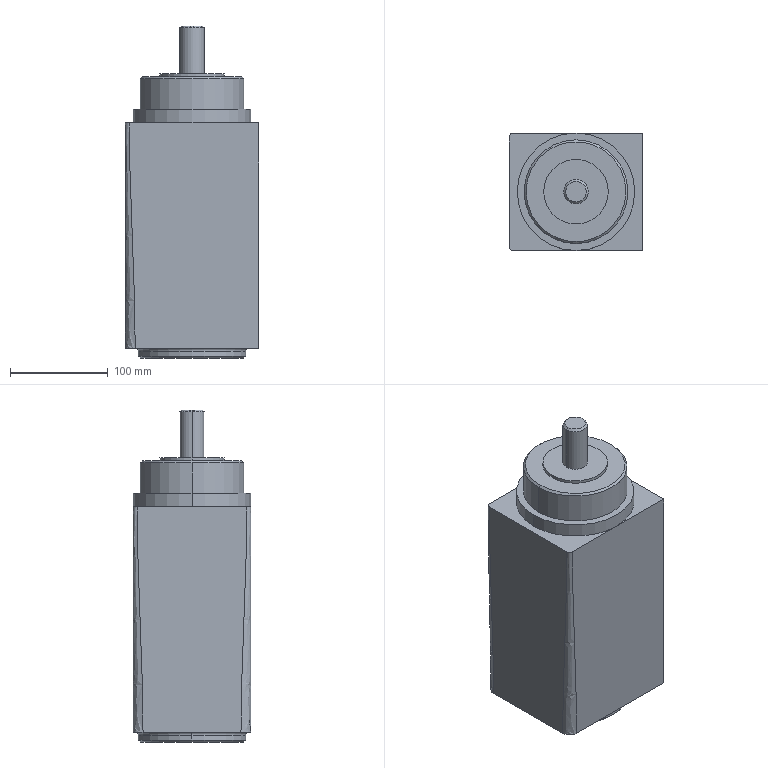Part | SolidWorks | features ICE 5, Chamfer 3, Extrusion 1, Fillet 1, VarFillet 1 | 1 solid | 32 faces | box 136 x 120 x 339 mm | volume 4326420 mm3 | plane 12 | cylinder 10 | cone 6 | torus 2 | spline 2 | commonest cylinder face diameters 25 x2 66 x2 106 x2 110 x2 120 x2
STEP:
#1=CARTESIAN_POINT('',(-53.,1.606,-240.));
#2=VERTEX_POINT('',#1);
#3=CARTESIAN_POINT('',(53.,1.606,-240.));
#4=VERTEX_POINT('',#3);
#5=CARTESIAN_POINT('',(0.,1.606,-240.));
#6=DIRECTION('',(0.,0.,-1.));
#7=DIRECTION('',(-1.,0.,0.));
#8=AXIS2_PLACEMENT_3D('',#5,#6,#7);
#9=CIRCLE('',#8,53.);
#10=EDGE_CURVE('',#2,#4,#9,.T.);
#11=ORIENTED_EDGE('',*,*,#10,.F.);
#12=CARTESIAN_POINT('',(-55.,1.606,-238.));
#13=VERTEX_POINT('',#12);
#14=CARTESIAN_POINT('',(-53.,1.606,-240.));
#15=DIRECTION('',(-0.7071,0.,0.7071));
#16=VECTOR('',#15,1000.);
#17=LINE('',#14,#16);
#18=EDGE_CURVE('',#2,#13,#17,.T.);
#19=ORIENTED_EDGE('',*,*,#18,.T.);
#20=CARTESIAN_POINT('',(55.,1.606,-238.));
#21=VERTEX_POINT('',#20);
#22=CARTESIAN_POINT('',(0.,1.606,-238.));
#23=DIRECTION('',(0.,0.,1.));
#24=DIRECTION('',(-1.,0.,0.));
#25=AXIS2_PLACEMENT_3D('',#22,#23,#24);
#26=CIRCLE('',#25,55.);
#27=EDGE_CURVE('',#21,#13,#26,.T.);
#28=ORIENTED_EDGE('',*,*,#27,.F.);
#29=CARTESIAN_POINT('',(53.,1.606,-240.));
#30=DIRECTION('',(0.7071,0.,0.7071));
#31=VECTOR('',#30,1000.);
#32=LINE('',#29,#31);
#33=EDGE_CURVE('',#4,#21,#32,.T.);
#34=ORIENTED_EDGE('',*,*,#33,.F.);
#35=EDGE_LOOP('',(#11,#19,#28,#34));
#36=FACE_OUTER_BOUND('',#35,.T.);
#37=CARTESIAN_POINT('',(0.,1.606,-240.));
#38=DIRECTION('',(0.,0.,1.));
#39=DIRECTION('',(1.,0.,0.));
#40=AXIS2_PLACEMENT_3D('',#37,#38,#39);
#41=CONICAL_SURFACE('',#40,53.,0.7854);
#42=ADVANCED_FACE('',(#36),#41,.T.);
#43=CARTESIAN_POINT('',(51.,1.606,47.));
#44=VERTEX_POINT('',#43);
#45=CARTESIAN_POINT('',(-51.,1.606,47.));
#46=VERTEX_POINT('',#45);
#47=CARTESIAN_POINT('',(0.,1.606,47.));
#48=DIRECTION('',(0.,0.,1.));
#49=DIRECTION('',(1.,0.,0.));
#50=AXIS2_PLACEMENT_3D('',#47,#48,#49);
#51=CIRCLE('',#50,51.);
#52=EDGE_CURVE('',#44,#46,#51,.T.);
#53=ORIENTED_EDGE('',*,*,#52,.F.);
#54=CARTESIAN_POINT('',(53.,1.606,45.));
#55=VERTEX_POINT('',#54);
#56=CARTESIAN_POINT('',(51.,1.606,47.));
#57=DIRECTION('',(0.7071,0.,-0.7071));
#58=VECTOR('',#57,1000.);
#59=LINE('',#56,#58);
#60=EDGE_CURVE('',#44,#55,#59,.T.);
#61=ORIENTED_EDGE('',*,*,#60,.T.);
#62=CARTESIAN_POINT('',(-53.,1.606,45.));
#63=VERTEX_POINT('',#62);
#64=CARTESIAN_POINT('',(0.,1.606,45.));
#65=DIRECTION('',(0.,0.,-1.));
#66=DIRECTION('',(1.,0.,0.));
#67=AXIS2_PLACEMENT_3D('',#64,#65,#66);
#68=CIRCLE('',#67,53.);
#69=EDGE_CURVE('',#63,#55,#68,.T.);
#70=ORIENTED_EDGE('',*,*,#69,.F.);
#71=CARTESIAN_POINT('',(-51.,1.606,47.));
#72=DIRECTION('',(-0.7071,0.,-0.7071));
#73=VECTOR('',#72,1000.);
#74=LINE('',#71,#73);
#75=EDGE_CURVE('',#46,#63,#74,.T.);
#76=ORIENTED_EDGE('',*,*,#75,.F.);
#77=EDGE_LOOP('',(#53,#61,#70,#76));
#78=FACE_OUTER_BOUND('',#77,.T.);
#79=CARTESIAN_POINT('',(0.,1.606,47.));
#80=DIRECTION('',(0.,0.,-1.));
#81=DIRECTION('',(-1.,0.,0.));
#82=AXIS2_PLACEMENT_3D('',#79,#80,#81);
#83=CONICAL_SURFACE('',#82,51.,0.7854);
#84=ADVANCED_FACE('',(#78),#83,.T.);
#85=CARTESIAN_POINT('',(-58.,1.606,-230.));
#86=VERTEX_POINT('',#85);
#87=CARTESIAN_POINT('',(58.,1.606,-230.));
#88=VERTEX_POINT('',#87);
#89=CARTESIAN_POINT('',(0.,1.606,-230.));
#90=DIRECTION('',(0.,0.,1.));
#91=DIRECTION('',(1.,0.,0.));
#92=AXIS2_PLACEMENT_3D('',#89,#90,#91);
#93=CIRCLE('',#92,58.);
#94=EDGE_CURVE('',#86,#88,#93,.T.);
#95=ORIENTED_EDGE('',*,*,#94,.F.);
#96=CARTESIAN_POINT('',(-55.,1.606,-233.));
#97=VERTEX_POINT('',#96);
#98=CARTESIAN_POINT('',(-58.,1.606,-233.));
#99=DIRECTION('',(0.,1.,0.));
#100=DIRECTION('',(-1.,0.,0.));
#101=AXIS2_PLACEMENT_3D('',#98,#99,#100);
#102=CIRCLE('',#101,3.);
#103=EDGE_CURVE('',#86,#97,#102,.T.);
#104=ORIENTED_EDGE('',*,*,#103,.T.);
#105=CARTESIAN_POINT('',(55.,1.606,-233.));
#106=VERTEX_POINT('',#105);
#107=CARTESIAN_POINT('',(0.,1.606,-233.));
#108=DIRECTION('',(0.,0.,-1.));
#109=DIRECTION('',(1.,0.,0.));
#110=AXIS2_PLACEMENT_3D('',#107,#108,#109);
#111=CIRCLE('',#110,55.);
#112=EDGE_CURVE('',#106,#97,#111,.T.);
#113=ORIENTED_EDGE('',*,*,#112,.F.);
#114=CARTESIAN_POINT('',(58.,1.606,-233.));
#115=DIRECTION('',(0.,-1.,0.));
#116=DIRECTION('',(0.,0.,-1.));
#117=AXIS2_PLACEMENT_3D('',#114,#115,#116);
#118=CIRCLE('',#117,3.);
#119=EDGE_CURVE('',#88,#106,#118,.T.);
#120=ORIENTED_EDGE('',*,*,#119,.F.);
#121=EDGE_LOOP('',(#95,#104,#113,#120));
#122=FACE_OUTER_BOUND('',#121,.T.);
#123=CARTESIAN_POINT('',(0.,1.606,-233.));
#124=DIRECTION('',(0.,0.,1.));
#125=DIRECTION('',(1.,0.,0.));
#126=AXIS2_PLACEMENT_3D('',#123,#124,#125);
#127=TOROIDAL_SURFACE('',#126,58.,3.);
#128=ADVANCED_FACE('',(#122),#127,.F.);
#129=ORIENTED_EDGE('',*,*,#27,.T.);
#130=CARTESIAN_POINT('',(-55.,1.606,-240.));
#131=DIRECTION('',(0.,0.,1.));
#132=VECTOR('',#131,1000.);
#133=LINE('',#130,#132);
#134=EDGE_CURVE('',#13,#97,#133,.T.);
#135=ORIENTED_EDGE('',*,*,#134,.T.);
#136=CARTESIAN_POINT('',(0.,1.606,-233.));
#137=DIRECTION('',(0.,0.,-1.));
#138=DIRECTION('',(1.,0.,0.));
#139=AXIS2_PLACEMENT_3D('',#136,#137,#138);
#140=CIRCLE('',#139,55.);
#141=EDGE_CURVE('',#97,#106,#140,.T.);
#142=ORIENTED_EDGE('',*,*,#141,.T.);
#143=CARTESIAN_POINT('',(55.,1.606,-240.));
#144=DIRECTION('',(0.,0.,1.));
#145=VECTOR('',#144,1000.);
#146=LINE('',#143,#145);
#147=EDGE_CURVE('',#21,#106,#146,.T.);
#148=ORIENTED_EDGE('',*,*,#147,.F.);
#149=EDGE_LOOP('',(#129,#135,#142,#148));
#150=FACE_OUTER_BOUND('',#149,.T.);
#151=CARTESIAN_POINT('',(0.,1.606,-240.));
#152=DIRECTION('',(0.,0.,1.));
#153=DIRECTION('',(1.,0.,0.));
#154=AXIS2_PLACEMENT_3D('',#151,#152,#153);
#155=CYLINDRICAL_SURFACE('',#154,55.);
#156=ADVANCED_FACE('',(#150),#155,.T.);
#157=CARTESIAN_POINT('',(10.5,1.606,99.));
#158=VERTEX_POINT('',#157);
#159=CARTESIAN_POINT('',(-10.5,1.606,99.));
#160=VERTEX_POINT('',#159);
#161=CARTESIAN_POINT('',(0.,1.606,99.));
#162=DIRECTION('',(0.,0.,1.));
#163=DIRECTION('',(1.,0.,0.));
#164=AXIS2_PLACEMENT_3D('',#161,#162,#163);
#165=CIRCLE('',#164,10.5);
#166=EDGE_CURVE('',#158,#160,#165,.T.);
#167=ORIENTED_EDGE('',*,*,#166,.F.);
#168=CARTESIAN_POINT('',(12.5,1.606,97.));
#169=VERTEX_POINT('',#168);
#170=CARTESIAN_POINT('',(10.5,1.606,99.));
#171=DIRECTION('',(0.7071,0.,-0.7071));
#172=VECTOR('',#171,1000.);
#173=LINE('',#170,#172);
#174=EDGE_CURVE('',#158,#169,#173,.T.);
#175=ORIENTED_EDGE('',*,*,#174,.T.);
#176=CARTESIAN_POINT('',(-12.5,1.606,97.));
#177=VERTEX_POINT('',#176);
#178=CARTESIAN_POINT('',(0.,1.606,97.));
#179=DIRECTION('',(0.,0.,-1.));
#180=DIRECTION('',(1.,0.,0.));
#181=AXIS2_PLACEMENT_3D('',#178,#179,#180);
#182=CIRCLE('',#181,12.5);
#183=EDGE_CURVE('',#177,#169,#182,.T.);
#184=ORIENTED_EDGE('',*,*,#183,.F.);
#185=CARTESIAN_POINT('',(-10.5,1.606,99.));
#186=DIRECTION('',(-0.7071,0.,-0.7071));
#187=VECTOR('',#186,1000.);
#188=LINE('',#185,#187);
#189=EDGE_CURVE('',#160,#177,#188,.T.);
#190=ORIENTED_EDGE('',*,*,#189,.F.);
#191=EDGE_LOOP('',(#167,#175,#184,#190));
#192=FACE_OUTER_BOUND('',#191,.T.);
#193=CARTESIAN_POINT('',(0.,1.606,99.));
#194=DIRECTION('',(0.,0.,-1.));
#195=DIRECTION('',(-1.,0.,0.));
#196=AXIS2_PLACEMENT_3D('',#193,#194,#195);
#197=CONICAL_SURFACE('',#196,10.5,0.7854);
#198=ADVANCED_FACE('',(#192),#197,.T.);
#199=ORIENTED_EDGE('',*,*,#183,.T.);
#200=CARTESIAN_POINT('',(12.5,1.606,50.));
#201=VERTEX_POINT('',#200);
#202=CARTESIAN_POINT('',(12.5,1.606,99.));
#203=DIRECTION('',(0.,0.,-1.));
#204=VECTOR('',#203,1000.);
#205=LINE('',#202,#204);
#206=EDGE_CURVE('',#169,#201,#205,.T.);
#207=ORIENTED_EDGE('',*,*,#206,.T.);
#208=CARTESIAN_POINT('',(-12.5,1.606,50.));
#209=VERTEX_POINT('',#208);
#210=CARTESIAN_POINT('',(0.,1.606,50.));
#211=DIRECTION('',(0.,0.,1.));
#212=DIRECTION('',(1.,0.,0.));
#213=AXIS2_PLACEMENT_3D('',#210,#211,#212);
#214=CIRCLE('',#213,12.5);
#215=EDGE_CURVE('',#201,#209,#214,.T.);
#216=ORIENTED_EDGE('',*,*,#215,.T.);
#217=CARTESIAN_POINT('',(-12.5,1.606,99.));
#218=DIRECTION('',(0.,0.,-1.));
#219=VECTOR('',#218,1000.);
#220=LINE('',#217,#219);
#221=EDGE_CURVE('',#177,#209,#220,.T.);
#222=ORIENTED_EDGE('',*,*,#221,.F.);
#223=EDGE_LOOP('',(#199,#207,#216,#222));
#224=FACE_OUTER_BOUND('',#223,.T.);
#225=CARTESIAN_POINT('',(0.,1.606,99.));
#226=DIRECTION('',(0.,0.,-1.));
#227=DIRECTION('',(-1.,0.,0.));
#228=AXIS2_PLACEMENT_3D('',#225,#226,#227);
#229=CYLINDRICAL_SURFACE('',#228,12.5);
#230=ADVANCED_FACE('',(#224),#229,.T.);
#231=CARTESIAN_POINT('',(33.,1.606,50.));
#232=VERTEX_POINT('',#231);
#233=CARTESIAN_POINT('',(-33.,1.606,50.));
#234=VERTEX_POINT('',#233);
#235=CARTESIAN_POINT('',(0.,1.606,50.));
#236=DIRECTION('',(0.,0.,1.));
#237=DIRECTION('',(1.,0.,0.));
#238=AXIS2_PLACEMENT_3D('',#235,#236,#237);
#239=CIRCLE('',#238,33.);
#240=EDGE_CURVE('',#232,#234,#239,.T.);
#241=ORIENTED_EDGE('',*,*,#240,.F.);
#242=CARTESIAN_POINT('',(33.,1.606,47.));
#243=VERTEX_POINT('',#242);
#244=CARTESIAN_POINT('',(33.,1.606,50.));
#245=DIRECTION('',(0.,0.,-1.));
#246=VECTOR('',#245,1000.);
#247=LINE('',#244,#246);
#248=EDGE_CURVE('',#232,#243,#247,.T.);
#249=ORIENTED_EDGE('',*,*,#248,.T.);
#250=CARTESIAN_POINT('',(-33.,1.606,47.));
#251=VERTEX_POINT('',#250);
#252=CARTESIAN_POINT('',(0.,1.606,47.));
#253=DIRECTION('',(0.,0.,1.));
#254=DIRECTION('',(1.,0.,0.));
#255=AXIS2_PLACEMENT_3D('',#252,#253,#254);
#256=CIRCLE('',#255,33.);
#257=EDGE_CURVE('',#243,#251,#256,.T.);
#258=ORIENTED_EDGE('',*,*,#257,.T.);
#259=CARTESIAN_POINT('',(-33.,1.606,50.));
#260=DIRECTION('',(0.,0.,-1.));
#261=VECTOR('',#260,1000.);
#262=LINE('',#259,#261);
#263=EDGE_CURVE('',#234,#251,#262,.T.);
#264=ORIENTED_EDGE('',*,*,#263,.F.);
#265=EDGE_LOOP('',(#241,#249,#258,#264));
#266=FACE_OUTER_BOUND('',#265,.T.);
#267=CARTESIAN_POINT('',(0.,1.606,50.));
#268=DIRECTION('',(0.,0.,-1.));
#269=DIRECTION('',(-1.,0.,0.));
#270=AXIS2_PLACEMENT_3D('',#267,#268,#269);
#271=CYLINDRICAL_SURFACE('',#270,33.);
#272=ADVANCED_FACE('',(#266),#271,.T.);
#273=ORIENTED_EDGE('',*,*,#69,.T.);
#274=CARTESIAN_POINT('',(53.,1.606,14.));
#275=VERTEX_POINT('',#274);
#276=CARTESIAN_POINT('',(53.,1.606,47.));
#277=DIRECTION('',(0.,0.,-1.));
#278=VECTOR('',#277,1000.);
#279=LINE('',#276,#278);
#280=EDGE_CURVE('',#55,#275,#279,.T.);
#281=ORIENTED_EDGE('',*,*,#280,.T.);
#282=CARTESIAN_POINT('',(-53.,1.606,14.));
#283=VERTEX_POINT('',#282);
#284=CARTESIAN_POINT('',(0.,1.606,14.));
#285=DIRECTION('',(0.,0.,1.));
#286=DIRECTION('',(1.,0.,0.));
#287=AXIS2_PLACEMENT_3D('',#284,#285,#286);
#288=CIRCLE('',#287,53.);
#289=EDGE_CURVE('',#275,#283,#288,.T.);
#290=ORIENTED_EDGE('',*,*,#289,.T.);
#291=CARTESIAN_POINT('',(-53.,1.606,47.));
#292=DIRECTION('',(0.,0.,-1.));
#293=VECTOR('',#292,1000.);
#294=LINE('',#291,#293);
#295=EDGE_CURVE('',#63,#283,#294,.T.);
#296=ORIENTED_EDGE('',*,*,#295,.F.);
#297=EDGE_LOOP('',(#273,#281,#290,#296));
#298=FACE_OUTER_BOUND('',#297,.T.);
#299=CARTESIAN_POINT('',(0.,1.606,47.));
#300=DIRECTION('',(0.,0.,-1.));
#301=DIRECTION('',(-1.,0.,0.));
#302=AXIS2_PLACEMENT_3D('',#299,#300,#301);
#303=CYLINDRICAL_SURFACE('',#302,53.);
#304=ADVANCED_FACE('',(#298),#303,.T.);
#305=CARTESIAN_POINT('',(60.,1.606,14.));
#306=VERTEX_POINT('',#305);
#307=CARTESIAN_POINT('',(-60.,1.606,14.));
#308=VERTEX_POINT('',#307);
#309=CARTESIAN_POINT('',(0.,1.606,14.));
#310=DIRECTION('',(0.,0.,1.));
#311=DIRECTION('',(1.,0.,0.));
#312=AXIS2_PLACEMENT_3D('',#309,#310,#311);
#313=CIRCLE('',#312,60.);
#314=EDGE_CURVE('',#306,#308,#313,.T.);
#315=ORIENTED_EDGE('',*,*,#314,.F.);
#316=CARTESIAN_POINT('',(60.,1.606,0.));
#317=VERTEX_POINT('',#316);
#318=CARTESIAN_POINT('',(60.,1.606,14.));
#319=DIRECTION('',(0.,0.,-1.));
#320=VECTOR('',#319,1000.);
#321=LINE('',#318,#320);
#322=EDGE_CURVE('',#306,#317,#321,.T.);
#323=ORIENTED_EDGE('',*,*,#322,.T.);
#324=CARTESIAN_POINT('',(0.,61.606,0.));
#325=VERTEX_POINT('',#324);
#326=CARTESIAN_POINT('',(0.,1.606,0.));
#327=DIRECTION('',(0.,0.,1.));
#328=DIRECTION('',(1.,0.,0.));
#329=AXIS2_PLACEMENT_3D('',#326,#327,#328);
#330=CIRCLE('',#329,60.);
#331=EDGE_CURVE('',#317,#325,#330,.T.);
#332=ORIENTED_EDGE('',*,*,#331,.T.);
#333=CARTESIAN_POINT('',(-60.,1.606,0.));
#334=VERTEX_POINT('',#333);
#335=CARTESIAN_POINT('',(0.,1.606,0.));
#336=DIRECTION('',(0.,0.,1.));
#337=DIRECTION('',(1.,0.,0.));
#338=AXIS2_PLACEMENT_3D('',#335,#336,#337);
#339=CIRCLE('',#338,60.);
#340=EDGE_CURVE('',#325,#334,#339,.T.);
#341=ORIENTED_EDGE('',*,*,#340,.T.);
#342=CARTESIAN_POINT('',(-60.,1.606,14.));
#343=DIRECTION('',(0.,0.,-1.));
#344=VECTOR('',#343,1000.);
#345=LINE('',#342,#344);
#346=EDGE_CURVE('',#308,#334,#345,.T.);
#347=ORIENTED_EDGE('',*,*,#346,.F.);
#348=EDGE_LOOP('',(#315,#323,#332,#341,#347));
#349=FACE_OUTER_BOUND('',#348,.T.);
#350=CARTESIAN_POINT('',(0.,1.606,14.));
#351=DIRECTION('',(0.,0.,-1.));
#352=DIRECTION('',(-1.,0.,0.));
#353=AXIS2_PLACEMENT_3D('',#350,#351,#352);
#354=CYLINDRICAL_SURFACE('',#353,60.);
#355=ADVANCED_FACE('',(#349),#354,.T.);
#356=CARTESIAN_POINT('',(-68.,57.606,0.));
#357=VERTEX_POINT('',#356);
#358=CARTESIAN_POINT('',(-68.,-54.394,0.));
#359=VERTEX_POINT('',#358);
#360=CARTESIAN_POINT('',(-68.,61.606,0.));
#361=DIRECTION('',(0.,-1.,0.));
#362=VECTOR('',#361,1000.);
#363=LINE('',#360,#362);
#364=EDGE_CURVE('',#357,#359,#363,.T.);
#365=ORIENTED_EDGE('',*,*,#364,.T.);
#366=CARTESIAN_POINT('',(-64.,-58.394,0.));
#367=VERTEX_POINT('',#366);
#368=CARTESIAN_POINT('',(-68.,-54.394,0.));
#369=CARTESIAN_POINT('',(-68.,-58.394,0.));
#370=CARTESIAN_POINT('',(-64.,-58.394,0.));
#371=(BOUNDED_CURVE()B_SPLINE_CURVE(2,(#368,#369,#370),.UNSPECIFIED.,.F.,.F.)B_SPLINE_CURVE_WITH_KNOTS((3,3),(0.,0.006249),.UNSPECIFIED.)CURVE()GEOMETRIC_REPRESENTATION_ITEM()RATIONAL_B_SPLINE_CURVE((1.,0.7071,1.))REPRESENTATION_ITEM(''));
#372=EDGE_CURVE('',#359,#367,#371,.T.);
#373=ORIENTED_EDGE('',*,*,#372,.T.);
#374=CARTESIAN_POINT('',(0.,-58.394,0.));
#375=VERTEX_POINT('',#374);
#376=CARTESIAN_POINT('',(-68.,-58.394,0.));
#377=DIRECTION('',(1.,0.,0.));
#378=VECTOR('',#377,1000.);
#379=LINE('',#376,#378);
#380=EDGE_CURVE('',#367,#375,#379,.T.);
#381=ORIENTED_EDGE('',*,*,#380,.T.);
#382=CARTESIAN_POINT('',(0.,1.606,0.));
#383=DIRECTION('',(0.,0.,1.));
#384=DIRECTION('',(1.,0.,0.));
#385=AXIS2_PLACEMENT_3D('',#382,#383,#384);
#386=CIRCLE('',#385,60.);
#387=EDGE_CURVE('',#334,#375,#386,.T.);
#388=ORIENTED_EDGE('',*,*,#387,.F.);
#389=ORIENTED_EDGE('',*,*,#340,.F.);
#390=CARTESIAN_POINT('',(-64.,61.606,0.));
#391=VERTEX_POINT('',#390);
#392=CARTESIAN_POINT('',(-68.,61.606,0.));
#393=DIRECTION('',(1.,0.,0.));
#394=VECTOR('',#393,1000.);
#395=LINE('',#392,#394);
#396=EDGE_CURVE('',#391,#325,#395,.T.);
#397=ORIENTED_EDGE('',*,*,#396,.F.);
#398=CARTESIAN_POINT('',(-64.,61.606,0.));
#399=CARTESIAN_POINT('',(-68.,61.606,0.));
#400=CARTESIAN_POINT('',(-68.,57.606,0.));
#401=(BOUNDED_CURVE()B_SPLINE_CURVE(2,(#398,#399,#400),.UNSPECIFIED.,.F.,.T.)B_SPLINE_CURVE_WITH_KNOTS((3,3),(0.,0.006249),.UNSPECIFIED.)CURVE()GEOMETRIC_REPRESENTATION_ITEM()RATIONAL_B_SPLINE_CURVE((1.,0.7071,1.))REPRESENTATION_ITEM(''));
#402=EDGE_CURVE('',#391,#357,#401,.T.);
#403=ORIENTED_EDGE('',*,*,#402,.T.);
#404=EDGE_LOOP('',(#365,#373,#381,#388,#389,#397,#403));
#405=FACE_OUTER_BOUND('',#404,.T.);
#406=CARTESIAN_POINT('',(0.,0.,0.));
#407=DIRECTION('',(0.,0.,1.));
#408=DIRECTION('',(1.,0.,0.));
#409=AXIS2_PLACEMENT_3D('',#406,#407,#408);
#410=PLANE('',#409);
#411=ADVANCED_FACE('',(#405),#410,.T.);
#412=CARTESIAN_POINT('',(-68.,51.606,-230.));
#413=VERTEX_POINT('',#412);
#414=CARTESIAN_POINT('',(-68.,-48.394,-230.));
#415=VERTEX_POINT('',#414);
#416=CARTESIAN_POINT('',(-68.,61.606,-230.));
#417=DIRECTION('',(0.,-1.,0.));
#418=VECTOR('',#417,1000.);
#419=LINE('',#416,#418);
#420=EDGE_CURVE('',#413,#415,#419,.T.);
#421=ORIENTED_EDGE('',*,*,#420,.T.);
#422=CARTESIAN_POINT('',(-68.,-48.394,-230.));
#423=CARTESIAN_POINT('',(-68.,-48.394,-153.333));
#424=CARTESIAN_POINT('',(-68.,-54.394,-76.667));
#425=CARTESIAN_POINT('',(-68.,-54.394,0.));
#426=B_SPLINE_CURVE_WITH_KNOTS('',3,(#422,#423,#424,#425),.UNSPECIFIED.,.F.,.F.,(4,4),(0.,0.23),.UNSPECIFIED.);
#427=EDGE_CURVE('',#415,#359,#426,.T.);
#428=ORIENTED_EDGE('',*,*,#427,.T.);
#429=ORIENTED_EDGE('',*,*,#364,.F.);
#430=CARTESIAN_POINT('',(-68.,57.606,0.));
#431=CARTESIAN_POINT('',(-68.,57.606,-76.667));
#432=CARTESIAN_POINT('',(-68.,51.606,-153.333));
#433=CARTESIAN_POINT('',(-68.,51.606,-230.));
#434=B_SPLINE_CURVE_WITH_KNOTS('',3,(#430,#431,#432,#433),.UNSPECIFIED.,.F.,.F.,(4,4),(0.,0.23),.UNSPECIFIED.);
#435=EDGE_CURVE('',#357,#413,#434,.T.);
#436=ORIENTED_EDGE('',*,*,#435,.T.);
#437=EDGE_LOOP('',(#421,#428,#429,#436));
#438=FACE_OUTER_BOUND('',#437,.T.);
#439=CARTESIAN_POINT('',(-68.,61.606,-230.));
#440=DIRECTION('',(-1.,0.,0.));
#441=DIRECTION('',(0.,0.,1.));
#442=AXIS2_PLACEMENT_3D('',#439,#440,#441);
#443=PLANE('',#442);
#444=ADVANCED_FACE('',(#438),#443,.T.);
#445=CARTESIAN_POINT('',(-58.,61.606,-230.));
#446=VERTEX_POINT('',#445);
#447=CARTESIAN_POINT('',(68.,61.606,-230.));
#448=VERTEX_POINT('',#447);
#449=CARTESIAN_POINT('',(-68.,61.606,-230.));
#450=DIRECTION('',(1.,0.,0.));
#451=VECTOR('',#450,1000.);
#452=LINE('',#449,#451);
#453=EDGE_CURVE('',#446,#448,#452,.T.);
#454=ORIENTED_EDGE('',*,*,#453,.F.);
#455=CARTESIAN_POINT('',(-58.,61.606,-230.));
#456=CARTESIAN_POINT('',(-58.,61.606,-153.333));
#457=CARTESIAN_POINT('',(-64.,61.606,-76.667));
#458=CARTESIAN_POINT('',(-64.,61.606,0.));
#459=B_SPLINE_CURVE_WITH_KNOTS('',3,(#455,#456,#457,#458),.UNSPECIFIED.,.F.,.F.,(4,4),(0.,0.23),.UNSPECIFIED.);
#460=EDGE_CURVE('',#446,#391,#459,.T.);
#461=ORIENTED_EDGE('',*,*,#460,.T.);
#462=ORIENTED_EDGE('',*,*,#396,.T.);
#463=CARTESIAN_POINT('',(68.,61.606,0.));
#464=VERTEX_POINT('',#463);
#465=CARTESIAN_POINT('',(-68.,61.606,0.));
#466=DIRECTION('',(1.,0.,0.));
#467=VECTOR('',#466,1000.);
#468=LINE('',#465,#467);
#469=EDGE_CURVE('',#325,#464,#468,.T.);
#470=ORIENTED_EDGE('',*,*,#469,.T.);
#471=CARTESIAN_POINT('',(68.,61.606,-230.));
#472=DIRECTION('',(0.,0.,1.));
#473=VECTOR('',#472,1000.);
#474=LINE('',#471,#473);
#475=EDGE_CURVE('',#448,#464,#474,.T.);
#476=ORIENTED_EDGE('',*,*,#475,.F.);
#477=EDGE_LOOP('',(#454,#461,#462,#470,#476));
#478=FACE_OUTER_BOUND('',#477,.T.);
#479=CARTESIAN_POINT('',(-68.,61.606,-230.));
#480=DIRECTION('',(0.,-1.,0.));
#481=DIRECTION('',(1.,0.,0.));
#482=AXIS2_PLACEMENT_3D('',#479,#480,#481);
#483=PLANE('',#482);
#484=ADVANCED_FACE('',(#478),#483,.F.);
#485=CARTESIAN_POINT('',(68.,-58.394,0.));
#486=VERTEX_POINT('',#485);
#487=CARTESIAN_POINT('',(68.,61.606,0.));
#488=DIRECTION('',(0.,-1.,0.));
#489=VECTOR('',#488,1000.);
#490=LINE('',#487,#489);
#491=EDGE_CURVE('',#464,#486,#490,.T.);
#492=ORIENTED_EDGE('',*,*,#491,.T.);
#493=CARTESIAN_POINT('',(68.,-58.394,-230.));
#494=VERTEX_POINT('',#493);
#495=CARTESIAN_POINT('',(68.,-58.394,-230.));
#496=DIRECTION('',(0.,0.,1.));
#497=VECTOR('',#496,1000.);
#498=LINE('',#495,#497);
#499=EDGE_CURVE('',#494,#486,#498,.T.);
#500=ORIENTED_EDGE('',*,*,#499,.F.);
#501=CARTESIAN_POINT('',(68.,61.606,-230.));
#502=DIRECTION('',(0.,-1.,0.));
#503=VECTOR('',#502,1000.);
#504=LINE('',#501,#503);
#505=EDGE_CURVE('',#448,#494,#504,.T.);
#506=ORIENTED_EDGE('',*,*,#505,.F.);
#507=ORIENTED_EDGE('',*,*,#475,.T.);
#508=EDGE_LOOP('',(#492,#500,#506,#507));
#509=FACE_OUTER_BOUND('',#508,.T.);
#510=CARTESIAN_POINT('',(68.,61.606,-230.));
#511=DIRECTION('',(-1.,0.,0.));
#512=DIRECTION('',(0.,0.,1.));
#513=AXIS2_PLACEMENT_3D('',#510,#511,#512);
#514=PLANE('',#513);
#515=ADVANCED_FACE('',(#509),#514,.F.);
#516=ORIENTED_EDGE('',*,*,#380,.F.);
#517=CARTESIAN_POINT('',(-58.,-58.394,-230.));
#518=VERTEX_POINT('',#517);
#519=CARTESIAN_POINT('',(-64.,-58.394,0.));
#520=CARTESIAN_POINT('',(-64.,-58.394,-76.667));
#521=CARTESIAN_POINT('',(-58.,-58.394,-153.333));
#522=CARTESIAN_POINT('',(-58.,-58.394,-230.));
#523=B_SPLINE_CURVE_WITH_KNOTS('',3,(#519,#520,#521,#522),.UNSPECIFIED.,.F.,.F.,(4,4),(0.,0.23),.UNSPECIFIED.);
#524=EDGE_CURVE('',#367,#518,#523,.T.);
#525=ORIENTED_EDGE('',*,*,#524,.T.);
#526=CARTESIAN_POINT('',(-68.,-58.394,-230.));
#527=DIRECTION('',(1.,0.,0.));
#528=VECTOR('',#527,1000.);
#529=LINE('',#526,#528);
#530=EDGE_CURVE('',#518,#494,#529,.T.);
#531=ORIENTED_EDGE('',*,*,#530,.T.);
#532=ORIENTED_EDGE('',*,*,#499,.T.);
#533=CARTESIAN_POINT('',(-68.,-58.394,0.));
#534=DIRECTION('',(1.,0.,0.));
#535=VECTOR('',#534,1000.);
#536=LINE('',#533,#535);
#537=EDGE_CURVE('',#375,#486,#536,.T.);
#538=ORIENTED_EDGE('',*,*,#537,.F.);
#539=EDGE_LOOP('',(#516,#525,#531,#532,#538));
#540=FACE_OUTER_BOUND('',#539,.T.);
#541=CARTESIAN_POINT('',(-68.,-58.394,-230.));
#542=DIRECTION('',(0.,-1.,0.));
#543=DIRECTION('',(0.,0.,-1.));
#544=AXIS2_PLACEMENT_3D('',#541,#542,#543);
#545=PLANE('',#544);
#546=ADVANCED_FACE('',(#540),#545,.T.);
#547=CARTESIAN_POINT('',(0.,1.606,-230.));
#548=DIRECTION('',(0.,0.,1.));
#549=DIRECTION('',(1.,0.,0.));
#550=AXIS2_PLACEMENT_3D('',#547,#548,#549);
#551=CIRCLE('',#550,58.);
#552=EDGE_CURVE('',#88,#86,#551,.T.);
#553=ORIENTED_EDGE('',*,*,#552,.T.);
#554=ORIENTED_EDGE('',*,*,#94,.T.);
#555=EDGE_LOOP('',(#553,#554));
#556=FACE_BOUND('',#555,.T.);
#557=ORIENTED_EDGE('',*,*,#530,.F.);
#558=CARTESIAN_POINT('',(-58.,-58.394,-230.));
#559=CARTESIAN_POINT('',(-68.,-58.394,-230.));
#560=CARTESIAN_POINT('',(-68.,-48.394,-230.));
#561=(BOUNDED_CURVE()B_SPLINE_CURVE(2,(#558,#559,#560),.UNSPECIFIED.,.F.,.F.)B_SPLINE_CURVE_WITH_KNOTS((3,3),(0.,0.01562),.UNSPECIFIED.)CURVE()GEOMETRIC_REPRESENTATION_ITEM()RATIONAL_B_SPLINE_CURVE((1.,0.7071,1.))REPRESENTATION_ITEM(''));
#562=EDGE_CURVE('',#518,#415,#561,.T.);
#563=ORIENTED_EDGE('',*,*,#562,.T.);
#564=ORIENTED_EDGE('',*,*,#420,.F.);
#565=CARTESIAN_POINT('',(-68.,51.606,-230.));
#566=CARTESIAN_POINT('',(-68.,61.606,-230.));
#567=CARTESIAN_POINT('',(-58.,61.606,-230.));
#568=(BOUNDED_CURVE()B_SPLINE_CURVE(2,(#565,#566,#567),.UNSPECIFIED.,.F.,.F.)B_SPLINE_CURVE_WITH_KNOTS((3,3),(0.,0.01562),.UNSPECIFIED.)CURVE()GEOMETRIC_REPRESENTATION_ITEM()RATIONAL_B_SPLINE_CURVE((1.,0.7071,1.))REPRESENTATION_ITEM(''));
#569=EDGE_CURVE('',#413,#446,#568,.T.);
#570=ORIENTED_EDGE('',*,*,#569,.T.);
#571=ORIENTED_EDGE('',*,*,#453,.T.);
#572=ORIENTED_EDGE('',*,*,#505,.T.);
#573=EDGE_LOOP('',(#557,#563,#564,#570,#571,#572));
#574=FACE_OUTER_BOUND('',#573,.T.);
#575=CARTESIAN_POINT('',(0.,0.,-230.));
#576=DIRECTION('',(0.,0.,1.));
#577=DIRECTION('',(1.,0.,0.));
#578=AXIS2_PLACEMENT_3D('',#575,#576,#577);
#579=PLANE('',#578);
#580=ADVANCED_FACE('',(#556,#574),#579,.F.);
#581=CARTESIAN_POINT('',(0.,1.606,0.));
#582=DIRECTION('',(0.,0.,1.));
#583=DIRECTION('',(1.,0.,0.));
#584=AXIS2_PLACEMENT_3D('',#581,#582,#583);
#585=CIRCLE('',#584,60.);
#586=EDGE_CURVE('',#375,#317,#585,.T.);
#587=ORIENTED_EDGE('',*,*,#586,.F.);
#588=ORIENTED_EDGE('',*,*,#537,.T.);
#589=ORIENTED_EDGE('',*,*,#491,.F.);
#590=ORIENTED_EDGE('',*,*,#469,.F.);
#591=ORIENTED_EDGE('',*,*,#331,.F.);
#592=EDGE_LOOP('',(#587,#588,#589,#590,#591));
#593=FACE_OUTER_BOUND('',#592,.T.);
#594=CARTESIAN_POINT('',(0.,0.,0.));
#595=DIRECTION('',(0.,0.,1.));
#596=DIRECTION('',(1.,0.,0.));
#597=AXIS2_PLACEMENT_3D('',#594,#595,#596);
#598=PLANE('',#597);
#599=ADVANCED_FACE('',(#593),#598,.T.);
#600=ORIENTED_EDGE('',*,*,#322,.F.);
#601=CARTESIAN_POINT('',(0.,1.606,14.));
#602=DIRECTION('',(0.,0.,1.));
#603=DIRECTION('',(1.,0.,0.));
#604=AXIS2_PLACEMENT_3D('',#601,#602,#603);
#605=CIRCLE('',#604,60.);
#606=EDGE_CURVE('',#308,#306,#605,.T.);
#607=ORIENTED_EDGE('',*,*,#606,.F.);
#608=ORIENTED_EDGE('',*,*,#346,.T.);
#609=ORIENTED_EDGE('',*,*,#387,.T.);
#610=ORIENTED_EDGE('',*,*,#586,.T.);
#611=EDGE_LOOP('',(#600,#607,#608,#609,#610));
#612=FACE_OUTER_BOUND('',#611,.T.);
#613=CARTESIAN_POINT('',(0.,1.606,14.));
#614=DIRECTION('',(0.,0.,-1.));
#615=DIRECTION('',(-1.,0.,0.));
#616=AXIS2_PLACEMENT_3D('',#613,#614,#615);
#617=CYLINDRICAL_SURFACE('',#616,60.);
#618=ADVANCED_FACE('',(#612),#617,.T.);
#619=CARTESIAN_POINT('',(0.,1.606,14.));
#620=DIRECTION('',(0.,0.,1.));
#621=DIRECTION('',(1.,0.,0.));
#622=AXIS2_PLACEMENT_3D('',#619,#620,#621);
#623=CIRCLE('',#622,53.);
#624=EDGE_CURVE('',#283,#275,#623,.T.);
#625=ORIENTED_EDGE('',*,*,#624,.F.);
#626=ORIENTED_EDGE('',*,*,#289,.F.);
#627=EDGE_LOOP('',(#625,#626));
#628=FACE_BOUND('',#627,.T.);
#629=ORIENTED_EDGE('',*,*,#606,.T.);
#630=ORIENTED_EDGE('',*,*,#314,.T.);
#631=EDGE_LOOP('',(#629,#630));
#632=FACE_OUTER_BOUND('',#631,.T.);
#633=CARTESIAN_POINT('',(0.,1.606,14.));
#634=DIRECTION('',(0.,0.,1.));
#635=DIRECTION('',(1.,0.,0.));
#636=AXIS2_PLACEMENT_3D('',#633,#634,#635);
#637=PLANE('',#636);
#638=ADVANCED_FACE('',(#628,#632),#637,.T.);
#639=ORIENTED_EDGE('',*,*,#280,.F.);
#640=CARTESIAN_POINT('',(0.,1.606,45.));
#641=DIRECTION('',(0.,0.,-1.));
#642=DIRECTION('',(1.,0.,0.));
#643=AXIS2_PLACEMENT_3D('',#640,#641,#642);
#644=CIRCLE('',#643,53.);
#645=EDGE_CURVE('',#55,#63,#644,.T.);
#646=ORIENTED_EDGE('',*,*,#645,.T.);
#647=ORIENTED_EDGE('',*,*,#295,.T.);
#648=ORIENTED_EDGE('',*,*,#624,.T.);
#649=EDGE_LOOP('',(#639,#646,#647,#648));
#650=FACE_OUTER_BOUND('',#649,.T.);
#651=CARTESIAN_POINT('',(0.,1.606,47.));
#652=DIRECTION('',(0.,0.,-1.));
#653=DIRECTION('',(-1.,0.,0.));
#654=AXIS2_PLACEMENT_3D('',#651,#652,#653);
#655=CYLINDRICAL_SURFACE('',#654,53.);
#656=ADVANCED_FACE('',(#650),#655,.T.);
#657=CARTESIAN_POINT('',(0.,1.606,47.));
#658=DIRECTION('',(0.,0.,1.));
#659=DIRECTION('',(1.,0.,0.));
#660=AXIS2_PLACEMENT_3D('',#657,#658,#659);
#661=CIRCLE('',#660,51.);
#662=EDGE_CURVE('',#46,#44,#661,.T.);
#663=ORIENTED_EDGE('',*,*,#662,.T.);
#664=ORIENTED_EDGE('',*,*,#52,.T.);
#665=EDGE_LOOP('',(#663,#664));
#666=FACE_OUTER_BOUND('',#665,.T.);
#667=CARTESIAN_POINT('',(0.,1.606,47.));
#668=DIRECTION('',(0.,0.,1.));
#669=DIRECTION('',(1.,0.,0.));
#670=AXIS2_PLACEMENT_3D('',#667,#668,#669);
#671=CIRCLE('',#670,33.);
#672=EDGE_CURVE('',#251,#243,#671,.T.);
#673=ORIENTED_EDGE('',*,*,#672,.F.);
#674=ORIENTED_EDGE('',*,*,#257,.F.);
#675=EDGE_LOOP('',(#673,#674));
#676=FACE_BOUND('',#675,.T.);
#677=CARTESIAN_POINT('',(0.,1.606,47.));
#678=DIRECTION('',(0.,0.,1.));
#679=DIRECTION('',(1.,0.,0.));
#680=AXIS2_PLACEMENT_3D('',#677,#678,#679);
#681=PLANE('',#680);
#682=ADVANCED_FACE('',(#666,#676),#681,.T.);
#683=ORIENTED_EDGE('',*,*,#248,.F.);
#684=CARTESIAN_POINT('',(0.,1.606,50.));
#685=DIRECTION('',(0.,0.,1.));
#686=DIRECTION('',(1.,0.,0.));
#687=AXIS2_PLACEMENT_3D('',#684,#685,#686);
#688=CIRCLE('',#687,33.);
#689=EDGE_CURVE('',#234,#232,#688,.T.);
#690=ORIENTED_EDGE('',*,*,#689,.F.);
#691=ORIENTED_EDGE('',*,*,#263,.T.);
#692=ORIENTED_EDGE('',*,*,#672,.T.);
#693=EDGE_LOOP('',(#683,#690,#691,#692));
#694=FACE_OUTER_BOUND('',#693,.T.);
#695=CARTESIAN_POINT('',(0.,1.606,50.));
#696=DIRECTION('',(0.,0.,-1.));
#697=DIRECTION('',(-1.,0.,0.));
#698=AXIS2_PLACEMENT_3D('',#695,#696,#697);
#699=CYLINDRICAL_SURFACE('',#698,33.);
#700=ADVANCED_FACE('',(#694),#699,.T.);
#701=CARTESIAN_POINT('',(0.,1.606,50.));
#702=DIRECTION('',(0.,0.,1.));
#703=DIRECTION('',(1.,0.,0.));
#704=AXIS2_PLACEMENT_3D('',#701,#702,#703);
#705=CIRCLE('',#704,12.5);
#706=EDGE_CURVE('',#209,#201,#705,.T.);
#707=ORIENTED_EDGE('',*,*,#706,.F.);
#708=ORIENTED_EDGE('',*,*,#215,.F.);
#709=EDGE_LOOP('',(#707,#708));
#710=FACE_BOUND('',#709,.T.);
#711=ORIENTED_EDGE('',*,*,#689,.T.);
#712=ORIENTED_EDGE('',*,*,#240,.T.);
#713=EDGE_LOOP('',(#711,#712));
#714=FACE_OUTER_BOUND('',#713,.T.);
#715=CARTESIAN_POINT('',(0.,1.606,50.));
#716=DIRECTION('',(0.,0.,1.));
#717=DIRECTION('',(1.,0.,0.));
#718=AXIS2_PLACEMENT_3D('',#715,#716,#717);
#719=PLANE('',#718);
#720=ADVANCED_FACE('',(#710,#714),#719,.T.);
#721=ORIENTED_EDGE('',*,*,#206,.F.);
#722=CARTESIAN_POINT('',(0.,1.606,97.));
#723=DIRECTION('',(0.,0.,-1.));
#724=DIRECTION('',(1.,0.,0.));
#725=AXIS2_PLACEMENT_3D('',#722,#723,#724);
#726=CIRCLE('',#725,12.5);
#727=EDGE_CURVE('',#169,#177,#726,.T.);
#728=ORIENTED_EDGE('',*,*,#727,.T.);
#729=ORIENTED_EDGE('',*,*,#221,.T.);
#730=ORIENTED_EDGE('',*,*,#706,.T.);
#731=EDGE_LOOP('',(#721,#728,#729,#730));
#732=FACE_OUTER_BOUND('',#731,.T.);
#733=CARTESIAN_POINT('',(0.,1.606,99.));
#734=DIRECTION('',(0.,0.,-1.));
#735=DIRECTION('',(-1.,0.,0.));
#736=AXIS2_PLACEMENT_3D('',#733,#734,#735);
#737=CYLINDRICAL_SURFACE('',#736,12.5);
#738=ADVANCED_FACE('',(#732),#737,.T.);
#739=CARTESIAN_POINT('',(0.,1.606,99.));
#740=DIRECTION('',(0.,0.,1.));
#741=DIRECTION('',(1.,0.,0.));
#742=AXIS2_PLACEMENT_3D('',#739,#740,#741);
#743=CIRCLE('',#742,10.5);
#744=EDGE_CURVE('',#160,#158,#743,.T.);
#745=ORIENTED_EDGE('',*,*,#744,.T.);
#746=ORIENTED_EDGE('',*,*,#166,.T.);
#747=EDGE_LOOP('',(#745,#746));
#748=FACE_OUTER_BOUND('',#747,.T.);
#749=CARTESIAN_POINT('',(0.,1.606,99.));
#750=DIRECTION('',(0.,0.,1.));
#751=DIRECTION('',(1.,0.,0.));
#752=AXIS2_PLACEMENT_3D('',#749,#750,#751);
#753=PLANE('',#752);
#754=ADVANCED_FACE('',(#748),#753,.T.);
#755=ORIENTED_EDGE('',*,*,#174,.F.);
#756=ORIENTED_EDGE('',*,*,#744,.F.);
#757=ORIENTED_EDGE('',*,*,#189,.T.);
#758=ORIENTED_EDGE('',*,*,#727,.F.);
#759=EDGE_LOOP('',(#755,#756,#757,#758));
#760=FACE_OUTER_BOUND('',#759,.T.);
#761=CARTESIAN_POINT('',(0.,1.606,99.));
#762=DIRECTION('',(0.,0.,-1.));
#763=DIRECTION('',(-1.,0.,0.));
#764=AXIS2_PLACEMENT_3D('',#761,#762,#763);
#765=CONICAL_SURFACE('',#764,10.5,0.7854);
#766=ADVANCED_FACE('',(#760),#765,.T.);
#767=ORIENTED_EDGE('',*,*,#134,.F.);
#768=CARTESIAN_POINT('',(0.,1.606,-238.));
#769=DIRECTION('',(0.,0.,1.));
#770=DIRECTION('',(-1.,0.,0.));
#771=AXIS2_PLACEMENT_3D('',#768,#769,#770);
#772=CIRCLE('',#771,55.);
#773=EDGE_CURVE('',#13,#21,#772,.T.);
#774=ORIENTED_EDGE('',*,*,#773,.T.);
#775=ORIENTED_EDGE('',*,*,#147,.T.);
#776=ORIENTED_EDGE('',*,*,#112,.T.);
#777=EDGE_LOOP('',(#767,#774,#775,#776));
#778=FACE_OUTER_BOUND('',#777,.T.);
#779=CARTESIAN_POINT('',(0.,1.606,-240.));
#780=DIRECTION('',(0.,0.,1.));
#781=DIRECTION('',(1.,0.,0.));
#782=AXIS2_PLACEMENT_3D('',#779,#780,#781);
#783=CYLINDRICAL_SURFACE('',#782,55.);
#784=ADVANCED_FACE('',(#778),#783,.T.);
#785=CARTESIAN_POINT('',(0.,1.606,-240.));
#786=DIRECTION('',(0.,0.,-1.));
#787=DIRECTION('',(-1.,0.,0.));
#788=AXIS2_PLACEMENT_3D('',#785,#786,#787);
#789=CIRCLE('',#788,53.);
#790=EDGE_CURVE('',#4,#2,#789,.T.);
#791=ORIENTED_EDGE('',*,*,#790,.T.);
#792=ORIENTED_EDGE('',*,*,#10,.T.);
#793=EDGE_LOOP('',(#791,#792));
#794=FACE_OUTER_BOUND('',#793,.T.);
#795=CARTESIAN_POINT('',(0.,1.606,-240.));
#796=DIRECTION('',(0.,0.,-1.));
#797=DIRECTION('',(-1.,0.,0.));
#798=AXIS2_PLACEMENT_3D('',#795,#796,#797);
#799=PLANE('',#798);
#800=ADVANCED_FACE('',(#794),#799,.T.);
#801=ORIENTED_EDGE('',*,*,#103,.F.);
#802=ORIENTED_EDGE('',*,*,#552,.F.);
#803=ORIENTED_EDGE('',*,*,#119,.T.);
#804=ORIENTED_EDGE('',*,*,#141,.F.);
#805=EDGE_LOOP('',(#801,#802,#803,#804));
#806=FACE_OUTER_BOUND('',#805,.T.);
#807=CARTESIAN_POINT('',(0.,1.606,-233.));
#808=DIRECTION('',(0.,0.,1.));
#809=DIRECTION('',(1.,0.,0.));
#810=AXIS2_PLACEMENT_3D('',#807,#808,#809);
#811=TOROIDAL_SURFACE('',#810,58.,3.);
#812=ADVANCED_FACE('',(#806),#811,.F.);
#813=ORIENTED_EDGE('',*,*,#562,.F.);
#814=ORIENTED_EDGE('',*,*,#524,.F.);
#815=ORIENTED_EDGE('',*,*,#372,.F.);
#816=ORIENTED_EDGE('',*,*,#427,.F.);
#817=EDGE_LOOP('',(#813,#814,#815,#816));
#818=FACE_OUTER_BOUND('',#817,.T.);
#819=CARTESIAN_POINT('',(-68.,-48.394,-276.));
#820=CARTESIAN_POINT('',(-68.,-48.394,-260.667));
#821=CARTESIAN_POINT('',(-68.,-48.394,-245.333));
#822=CARTESIAN_POINT('',(-68.,-48.394,-230.));
#823=CARTESIAN_POINT('',(-68.,-48.394,-153.333));
#824=CARTESIAN_POINT('',(-68.,-54.394,-76.667));
#825=CARTESIAN_POINT('',(-68.,-54.394,0.));
#826=CARTESIAN_POINT('',(-68.,-54.394,15.333));
#827=CARTESIAN_POINT('',(-68.,-54.394,30.667));
#828=CARTESIAN_POINT('',(-68.,-54.394,46.));
#829=CARTESIAN_POINT('',(-68.,-58.394,-276.));
#830=CARTESIAN_POINT('',(-68.,-58.394,-260.667));
#831=CARTESIAN_POINT('',(-68.,-58.394,-245.333));
#832=CARTESIAN_POINT('',(-68.,-58.394,-230.));
#833=CARTESIAN_POINT('',(-68.,-58.394,-153.333));
#834=CARTESIAN_POINT('',(-68.,-58.394,-76.667));
#835=CARTESIAN_POINT('',(-68.,-58.394,0.));
#836=CARTESIAN_POINT('',(-68.,-58.394,15.333));
#837=CARTESIAN_POINT('',(-68.,-58.394,30.667));
#838=CARTESIAN_POINT('',(-68.,-58.394,46.));
#839=CARTESIAN_POINT('',(-58.,-58.394,-276.));
#840=CARTESIAN_POINT('',(-58.,-58.394,-260.667));
#841=CARTESIAN_POINT('',(-58.,-58.394,-245.333));
#842=CARTESIAN_POINT('',(-58.,-58.394,-230.));
#843=CARTESIAN_POINT('',(-58.,-58.394,-153.333));
#844=CARTESIAN_POINT('',(-64.,-58.394,-76.667));
#845=CARTESIAN_POINT('',(-64.,-58.394,0.));
#846=CARTESIAN_POINT('',(-64.,-58.394,15.333));
#847=CARTESIAN_POINT('',(-64.,-58.394,30.667));
#848=CARTESIAN_POINT('',(-64.,-58.394,46.));
#849=(BOUNDED_SURFACE()B_SPLINE_SURFACE(2,3,((#819,#820,#821,#822,#823,#824,#825,#826,#827,#828),(#829,#830,#831,#832,#833,#834,#835,#836,#837,#838),(#839,#840,#841,#842,#843,#844,#845,#846,#847,#848)),.UNSPECIFIED.,.F.,.F.,.F.)B_SPLINE_SURFACE_WITH_KNOTS((3,3),(4,3,3,4),(0.,1.),(-0.046,0.,0.23,0.276),.UNSPECIFIED.)GEOMETRIC_REPRESENTATION_ITEM()RATIONAL_B_SPLINE_SURFACE(((1.,1.,1.,1.,1.,1.,1.,1.,1.,1.),(0.7071,0.7071,0.7071,0.7071,0.7071,0.7071,0.7071,0.7071,0.7071,0.7071),(1.,1.,1.,1.,1.,1.,1.,1.,1.,1.)))REPRESENTATION_ITEM('')SURFACE());
#850=ADVANCED_FACE('',(#818),#849,.T.);
#851=ORIENTED_EDGE('',*,*,#569,.F.);
#852=ORIENTED_EDGE('',*,*,#435,.F.);
#853=ORIENTED_EDGE('',*,*,#402,.F.);
#854=ORIENTED_EDGE('',*,*,#460,.F.);
#855=EDGE_LOOP('',(#851,#852,#853,#854));
#856=FACE_OUTER_BOUND('',#855,.T.);
#857=CARTESIAN_POINT('',(-58.,61.606,-276.));
#858=CARTESIAN_POINT('',(-58.,61.606,-260.667));
#859=CARTESIAN_POINT('',(-58.,61.606,-245.333));
#860=CARTESIAN_POINT('',(-58.,61.606,-230.));
#861=CARTESIAN_POINT('',(-58.,61.606,-153.333));
#862=CARTESIAN_POINT('',(-64.,61.606,-76.667));
#863=CARTESIAN_POINT('',(-64.,61.606,0.));
#864=CARTESIAN_POINT('',(-64.,61.606,15.333));
#865=CARTESIAN_POINT('',(-64.,61.606,30.667));
#866=CARTESIAN_POINT('',(-64.,61.606,46.));
#867=CARTESIAN_POINT('',(-68.,61.606,-276.));
#868=CARTESIAN_POINT('',(-68.,61.606,-260.667));
#869=CARTESIAN_POINT('',(-68.,61.606,-245.333));
#870=CARTESIAN_POINT('',(-68.,61.606,-230.));
#871=CARTESIAN_POINT('',(-68.,61.606,-153.333));
#872=CARTESIAN_POINT('',(-68.,61.606,-76.667));
#873=CARTESIAN_POINT('',(-68.,61.606,0.));
#874=CARTESIAN_POINT('',(-68.,61.606,15.333));
#875=CARTESIAN_POINT('',(-68.,61.606,30.667));
#876=CARTESIAN_POINT('',(-68.,61.606,46.));
#877=CARTESIAN_POINT('',(-68.,51.606,-276.));
#878=CARTESIAN_POINT('',(-68.,51.606,-260.667));
#879=CARTESIAN_POINT('',(-68.,51.606,-245.333));
#880=CARTESIAN_POINT('',(-68.,51.606,-230.));
#881=CARTESIAN_POINT('',(-68.,51.606,-153.333));
#882=CARTESIAN_POINT('',(-68.,57.606,-76.667));
#883=CARTESIAN_POINT('',(-68.,57.606,0.));
#884=CARTESIAN_POINT('',(-68.,57.606,15.333));
#885=CARTESIAN_POINT('',(-68.,57.606,30.667));
#886=CARTESIAN_POINT('',(-68.,57.606,46.));
#887=(BOUNDED_SURFACE()B_SPLINE_SURFACE(2,3,((#857,#858,#859,#860,#861,#862,#863,#864,#865,#866),(#867,#868,#869,#870,#871,#872,#873,#874,#875,#876),(#877,#878,#879,#880,#881,#882,#883,#884,#885,#886)),.UNSPECIFIED.,.F.,.F.,.F.)B_SPLINE_SURFACE_WITH_KNOTS((3,3),(4,3,3,4),(0.,1.),(-0.046,0.,0.23,0.276),.UNSPECIFIED.)GEOMETRIC_REPRESENTATION_ITEM()RATIONAL_B_SPLINE_SURFACE(((1.,1.,1.,1.,1.,1.,1.,1.,1.,1.),(0.7071,0.7071,0.7071,0.7071,0.7071,0.7071,0.7071,0.7071,0.7071,0.7071),(1.,1.,1.,1.,1.,1.,1.,1.,1.,1.)))REPRESENTATION_ITEM('')SURFACE());
#888=ADVANCED_FACE('',(#856),#887,.T.);
#889=ORIENTED_EDGE('',*,*,#60,.F.);
#890=ORIENTED_EDGE('',*,*,#662,.F.);
#891=ORIENTED_EDGE('',*,*,#75,.T.);
#892=ORIENTED_EDGE('',*,*,#645,.F.);
#893=EDGE_LOOP('',(#889,#890,#891,#892));
#894=FACE_OUTER_BOUND('',#893,.T.);
#895=CARTESIAN_POINT('',(0.,1.606,47.));
#896=DIRECTION('',(0.,0.,-1.));
#897=DIRECTION('',(-1.,0.,0.));
#898=AXIS2_PLACEMENT_3D('',#895,#896,#897);
#899=CONICAL_SURFACE('',#898,51.,0.7854);
#900=ADVANCED_FACE('',(#894),#899,.T.);
#901=ORIENTED_EDGE('',*,*,#18,.F.);
#902=ORIENTED_EDGE('',*,*,#790,.F.);
#903=ORIENTED_EDGE('',*,*,#33,.T.);
#904=ORIENTED_EDGE('',*,*,#773,.F.);
#905=EDGE_LOOP('',(#901,#902,#903,#904));
#906=FACE_OUTER_BOUND('',#905,.T.);
#907=CARTESIAN_POINT('',(0.,1.606,-240.));
#908=DIRECTION('',(0.,0.,1.));
#909=DIRECTION('',(1.,0.,0.));
#910=AXIS2_PLACEMENT_3D('',#907,#908,#909);
#911=CONICAL_SURFACE('',#910,53.,0.7854);
#912=ADVANCED_FACE('',(#906),#911,.T.);
#913=CLOSED_SHELL('',(#42,#84,#128,#156,#198,#230,#272,#304,#355,#411,#444,#484,#515,#546,#580,#599,#618,#638,#656,#682,#700,#720,#738,#754,#766,#784,#800,#812,#850,#888,#900,#912));
#914=MANIFOLD_SOLID_BREP('',#913);
#915=CARTESIAN_POINT('',(0.,0.,0.));
#916=DIRECTION('',(0.,0.,1.));
#917=DIRECTION('',(1.,0.,0.));
#918=AXIS2_PLACEMENT_3D('',#915,#916,#917);
#919=(LENGTH_UNIT()NAMED_UNIT(*)SI_UNIT(.MILLI.,.METRE.));
#920=UNCERTAINTY_MEASURE_WITH_UNIT(LENGTH_MEASURE(0.00001),#919,'','');
#921=(NAMED_UNIT(*)PLANE_ANGLE_UNIT()SI_UNIT($,.RADIAN.));
#922=(NAMED_UNIT(*)SI_UNIT($,.STERADIAN.)SOLID_ANGLE_UNIT());
#923=(GEOMETRIC_REPRESENTATION_CONTEXT(3)GLOBAL_UNCERTAINTY_ASSIGNED_CONTEXT((#920))GLOBAL_UNIT_ASSIGNED_CONTEXT((#919,#921,#922))REPRESENTATION_CONTEXT('',''));
#924=ADVANCED_BREP_SHAPE_REPRESENTATION('',(#914,#918),#923);